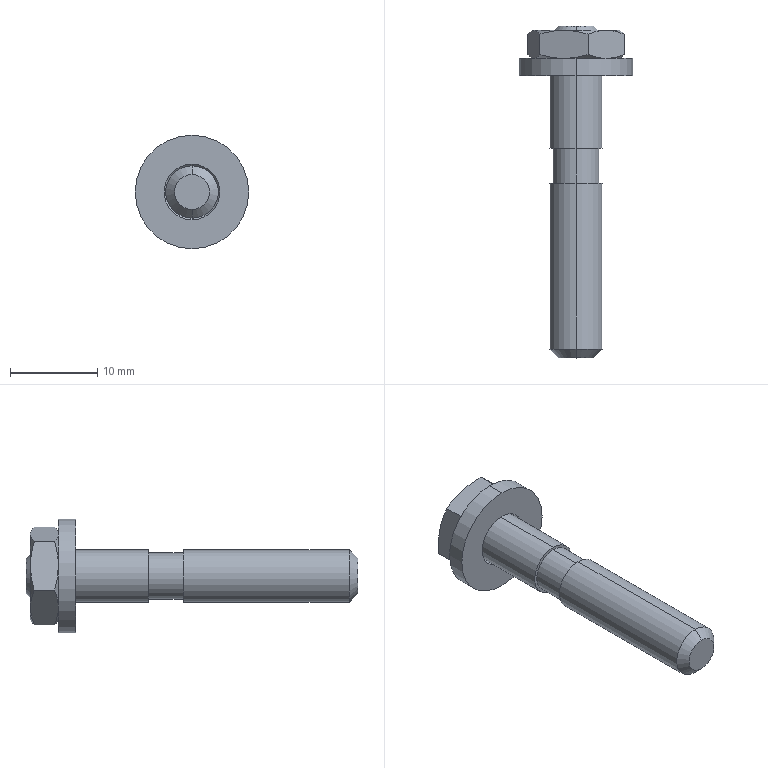Part | SolidWorks | features BaseBody 1 | 1 solid | 49 faces | box 13 x 38 x 13 mm | volume 1413 mm3 | cone 25 | plane 14 | cylinder 10 | commonest cylinder face diameters 6 x4 5.3 x2 6.4 x2 13 x2
STEP:
#1=CARTESIAN_POINT('',(13.099,44.62,-33.));
#2=VERTEX_POINT('',#1);
#3=CARTESIAN_POINT('',(13.099,44.62,-27.));
#4=VERTEX_POINT('',#3);
#5=CARTESIAN_POINT('',(13.099,44.62,-30.));
#6=DIRECTION('',(0.,-1.,0.));
#7=DIRECTION('',(0.,0.,-1.));
#8=AXIS2_PLACEMENT_3D('',#5,#6,#7);
#9=CIRCLE('',#8,3.);
#10=EDGE_CURVE('',#2,#4,#9,.T.);
#11=ORIENTED_EDGE('',*,*,#10,.T.);
#12=CARTESIAN_POINT('',(13.099,25.62,-27.));
#13=VERTEX_POINT('',#12);
#14=CARTESIAN_POINT('',(13.099,44.62,-27.));
#15=DIRECTION('',(0.,-1.,0.));
#16=VECTOR('',#15,1000.);
#17=LINE('',#14,#16);
#18=EDGE_CURVE('',#4,#13,#17,.T.);
#19=ORIENTED_EDGE('',*,*,#18,.T.);
#20=CARTESIAN_POINT('',(13.099,25.62,-33.));
#21=VERTEX_POINT('',#20);
#22=CARTESIAN_POINT('',(13.099,25.62,-30.));
#23=DIRECTION('',(0.,1.,0.));
#24=DIRECTION('',(0.,0.,-1.));
#25=AXIS2_PLACEMENT_3D('',#22,#23,#24);
#26=CIRCLE('',#25,3.);
#27=EDGE_CURVE('',#13,#21,#26,.T.);
#28=ORIENTED_EDGE('',*,*,#27,.T.);
#29=CARTESIAN_POINT('',(13.099,44.62,-33.));
#30=DIRECTION('',(0.,-1.,0.));
#31=VECTOR('',#30,1000.);
#32=LINE('',#29,#31);
#33=EDGE_CURVE('',#2,#21,#32,.T.);
#34=ORIENTED_EDGE('',*,*,#33,.F.);
#35=EDGE_LOOP('',(#11,#19,#28,#34));
#36=FACE_OUTER_BOUND('',#35,.T.);
#37=CARTESIAN_POINT('',(13.099,44.62,-30.));
#38=DIRECTION('',(0.,-1.,0.));
#39=DIRECTION('',(0.,0.,-1.));
#40=AXIS2_PLACEMENT_3D('',#37,#38,#39);
#41=CYLINDRICAL_SURFACE('',#40,3.);
#42=ADVANCED_FACE('',(#36),#41,.T.);
#43=CARTESIAN_POINT('',(13.099,24.62,-28.));
#44=VERTEX_POINT('',#43);
#45=CARTESIAN_POINT('',(13.099,24.62,-32.));
#46=VERTEX_POINT('',#45);
#47=CARTESIAN_POINT('',(13.099,24.62,-30.));
#48=DIRECTION('',(0.,1.,0.));
#49=DIRECTION('',(0.,0.,1.));
#50=AXIS2_PLACEMENT_3D('',#47,#48,#49);
#51=CIRCLE('',#50,2.);
#52=EDGE_CURVE('',#44,#46,#51,.T.);
#53=ORIENTED_EDGE('',*,*,#52,.T.);
#54=CARTESIAN_POINT('',(13.099,25.62,-33.));
#55=DIRECTION('',(0.,0.7071,-0.7071));
#56=VECTOR('',#55,1000.);
#57=LINE('',#54,#56);
#58=EDGE_CURVE('',#46,#21,#57,.T.);
#59=ORIENTED_EDGE('',*,*,#58,.T.);
#60=ORIENTED_EDGE('',*,*,#27,.F.);
#61=CARTESIAN_POINT('',(13.099,25.62,-27.));
#62=DIRECTION('',(0.,0.7071,0.7071));
#63=VECTOR('',#62,1000.);
#64=LINE('',#61,#63);
#65=EDGE_CURVE('',#44,#13,#64,.T.);
#66=ORIENTED_EDGE('',*,*,#65,.F.);
#67=EDGE_LOOP('',(#53,#59,#60,#66));
#68=FACE_OUTER_BOUND('',#67,.T.);
#69=CARTESIAN_POINT('',(13.099,25.62,-30.));
#70=DIRECTION('',(0.,1.,0.));
#71=DIRECTION('',(0.,0.,1.));
#72=AXIS2_PLACEMENT_3D('',#69,#70,#71);
#73=CONICAL_SURFACE('',#72,3.,0.7854);
#74=ADVANCED_FACE('',(#68),#73,.T.);
#75=CARTESIAN_POINT('',(13.099,48.62,-32.65));
#76=VERTEX_POINT('',#75);
#77=CARTESIAN_POINT('',(13.099,48.62,-27.35));
#78=VERTEX_POINT('',#77);
#79=CARTESIAN_POINT('',(13.099,48.62,-30.));
#80=DIRECTION('',(0.,-1.,0.));
#81=DIRECTION('',(0.,0.,-1.));
#82=AXIS2_PLACEMENT_3D('',#79,#80,#81);
#83=CIRCLE('',#82,2.65);
#84=EDGE_CURVE('',#76,#78,#83,.T.);
#85=ORIENTED_EDGE('',*,*,#84,.T.);
#86=CARTESIAN_POINT('',(13.099,44.62,-27.35));
#87=VERTEX_POINT('',#86);
#88=CARTESIAN_POINT('',(13.099,48.62,-27.35));
#89=DIRECTION('',(0.,-1.,0.));
#90=VECTOR('',#89,1000.);
#91=LINE('',#88,#90);
#92=EDGE_CURVE('',#78,#87,#91,.T.);
#93=ORIENTED_EDGE('',*,*,#92,.T.);
#94=CARTESIAN_POINT('',(13.099,44.62,-32.65));
#95=VERTEX_POINT('',#94);
#96=CARTESIAN_POINT('',(13.099,44.62,-30.));
#97=DIRECTION('',(0.,-1.,0.));
#98=DIRECTION('',(0.,0.,-1.));
#99=AXIS2_PLACEMENT_3D('',#96,#97,#98);
#100=CIRCLE('',#99,2.65);
#101=EDGE_CURVE('',#95,#87,#100,.T.);
#102=ORIENTED_EDGE('',*,*,#101,.F.);
#103=CARTESIAN_POINT('',(13.099,48.62,-32.65));
#104=DIRECTION('',(0.,-1.,0.));
#105=VECTOR('',#104,1000.);
#106=LINE('',#103,#105);
#107=EDGE_CURVE('',#76,#95,#106,.T.);
#108=ORIENTED_EDGE('',*,*,#107,.F.);
#109=EDGE_LOOP('',(#85,#93,#102,#108));
#110=FACE_OUTER_BOUND('',#109,.T.);
#111=CARTESIAN_POINT('',(13.099,48.62,-30.));
#112=DIRECTION('',(0.,-1.,0.));
#113=DIRECTION('',(0.,0.,-1.));
#114=AXIS2_PLACEMENT_3D('',#111,#112,#113);
#115=CYLINDRICAL_SURFACE('',#114,2.65);
#116=ADVANCED_FACE('',(#110),#115,.T.);
#117=CARTESIAN_POINT('',(13.099,59.42,-33.));
#118=VERTEX_POINT('',#117);
#119=CARTESIAN_POINT('',(13.099,59.42,-27.));
#120=VERTEX_POINT('',#119);
#121=CARTESIAN_POINT('',(13.099,59.42,-30.));
#122=DIRECTION('',(0.,-1.,0.));
#123=DIRECTION('',(0.,0.,-1.));
#124=AXIS2_PLACEMENT_3D('',#121,#122,#123);
#125=CIRCLE('',#124,3.);
#126=EDGE_CURVE('',#118,#120,#125,.T.);
#127=ORIENTED_EDGE('',*,*,#126,.T.);
#128=CARTESIAN_POINT('',(13.099,48.62,-27.));
#129=VERTEX_POINT('',#128);
#130=CARTESIAN_POINT('',(13.099,59.42,-27.));
#131=DIRECTION('',(0.,-1.,0.));
#132=VECTOR('',#131,1000.);
#133=LINE('',#130,#132);
#134=EDGE_CURVE('',#120,#129,#133,.T.);
#135=ORIENTED_EDGE('',*,*,#134,.T.);
#136=CARTESIAN_POINT('',(13.099,48.62,-33.));
#137=VERTEX_POINT('',#136);
#138=CARTESIAN_POINT('',(13.099,48.62,-30.));
#139=DIRECTION('',(0.,1.,0.));
#140=DIRECTION('',(0.,0.,-1.));
#141=AXIS2_PLACEMENT_3D('',#138,#139,#140);
#142=CIRCLE('',#141,3.);
#143=EDGE_CURVE('',#129,#137,#142,.T.);
#144=ORIENTED_EDGE('',*,*,#143,.T.);
#145=CARTESIAN_POINT('',(13.099,59.42,-33.));
#146=DIRECTION('',(0.,-1.,0.));
#147=VECTOR('',#146,1000.);
#148=LINE('',#145,#147);
#149=EDGE_CURVE('',#118,#137,#148,.T.);
#150=ORIENTED_EDGE('',*,*,#149,.F.);
#151=EDGE_LOOP('',(#127,#135,#144,#150));
#152=FACE_OUTER_BOUND('',#151,.T.);
#153=CARTESIAN_POINT('',(13.099,59.42,-30.));
#154=DIRECTION('',(0.,-1.,0.));
#155=DIRECTION('',(0.,0.,-1.));
#156=AXIS2_PLACEMENT_3D('',#153,#154,#155);
#157=CYLINDRICAL_SURFACE('',#156,3.);
#158=ADVANCED_FACE('',(#152),#157,.T.);
#159=CARTESIAN_POINT('',(13.099,59.42,-30.));
#160=DIRECTION('',(0.,-1.,0.));
#161=DIRECTION('',(0.,0.,-1.));
#162=AXIS2_PLACEMENT_3D('',#159,#160,#161);
#163=CIRCLE('',#162,3.);
#164=EDGE_CURVE('',#120,#118,#163,.T.);
#165=ORIENTED_EDGE('',*,*,#164,.F.);
#166=CARTESIAN_POINT('',(13.099,58.92,-26.5));
#167=VERTEX_POINT('',#166);
#168=CARTESIAN_POINT('',(13.099,58.92,-26.5));
#169=DIRECTION('',(0.,-0.7071,0.7071));
#170=VECTOR('',#169,1000.);
#171=LINE('',#168,#170);
#172=EDGE_CURVE('',#120,#167,#171,.T.);
#173=ORIENTED_EDGE('',*,*,#172,.T.);
#174=CARTESIAN_POINT('',(13.099,58.92,-33.5));
#175=VERTEX_POINT('',#174);
#176=CARTESIAN_POINT('',(13.099,58.92,-30.));
#177=DIRECTION('',(0.,1.,0.));
#178=DIRECTION('',(0.,0.,-1.));
#179=AXIS2_PLACEMENT_3D('',#176,#177,#178);
#180=CIRCLE('',#179,3.5);
#181=EDGE_CURVE('',#175,#167,#180,.T.);
#182=ORIENTED_EDGE('',*,*,#181,.F.);
#183=CARTESIAN_POINT('',(13.099,58.92,-33.5));
#184=DIRECTION('',(0.,-0.7071,-0.7071));
#185=VECTOR('',#184,1000.);
#186=LINE('',#183,#185);
#187=EDGE_CURVE('',#118,#175,#186,.T.);
#188=ORIENTED_EDGE('',*,*,#187,.F.);
#189=EDGE_LOOP('',(#165,#173,#182,#188));
#190=FACE_OUTER_BOUND('',#189,.T.);
#191=CARTESIAN_POINT('',(13.099,58.92,-30.));
#192=DIRECTION('',(0.,-1.,0.));
#193=DIRECTION('',(0.,0.,-1.));
#194=AXIS2_PLACEMENT_3D('',#191,#192,#193);
#195=CONICAL_SURFACE('',#194,3.5,0.7854);
#196=ADVANCED_FACE('',(#190),#195,.F.);
#197=CARTESIAN_POINT('',(13.099,56.92,-33.2));
#198=VERTEX_POINT('',#197);
#199=CARTESIAN_POINT('',(13.099,56.92,-26.8));
#200=VERTEX_POINT('',#199);
#201=CARTESIAN_POINT('',(13.099,56.92,-30.));
#202=DIRECTION('',(0.,1.,0.));
#203=DIRECTION('',(0.,0.,1.));
#204=AXIS2_PLACEMENT_3D('',#201,#202,#203);
#205=CIRCLE('',#204,3.2);
#206=EDGE_CURVE('',#198,#200,#205,.T.);
#207=ORIENTED_EDGE('',*,*,#206,.F.);
#208=CARTESIAN_POINT('',(13.099,58.92,-33.2));
#209=VERTEX_POINT('',#208);
#210=CARTESIAN_POINT('',(13.099,56.92,-33.2));
#211=DIRECTION('',(0.,1.,0.));
#212=VECTOR('',#211,1000.);
#213=LINE('',#210,#212);
#214=EDGE_CURVE('',#198,#209,#213,.T.);
#215=ORIENTED_EDGE('',*,*,#214,.T.);
#216=CARTESIAN_POINT('',(13.099,58.92,-26.8));
#217=VERTEX_POINT('',#216);
#218=CARTESIAN_POINT('',(13.099,58.92,-30.));
#219=DIRECTION('',(0.,-1.,0.));
#220=DIRECTION('',(0.,0.,1.));
#221=AXIS2_PLACEMENT_3D('',#218,#219,#220);
#222=CIRCLE('',#221,3.2);
#223=EDGE_CURVE('',#217,#209,#222,.T.);
#224=ORIENTED_EDGE('',*,*,#223,.F.);
#225=CARTESIAN_POINT('',(13.099,56.92,-26.8));
#226=DIRECTION('',(0.,1.,0.));
#227=VECTOR('',#226,1000.);
#228=LINE('',#225,#227);
#229=EDGE_CURVE('',#200,#217,#228,.T.);
#230=ORIENTED_EDGE('',*,*,#229,.F.);
#231=EDGE_LOOP('',(#207,#215,#224,#230));
#232=FACE_OUTER_BOUND('',#231,.T.);
#233=CARTESIAN_POINT('',(13.099,56.92,-30.));
#234=DIRECTION('',(0.,1.,0.));
#235=DIRECTION('',(0.,0.,1.));
#236=AXIS2_PLACEMENT_3D('',#233,#234,#235);
#237=CYLINDRICAL_SURFACE('',#236,3.2);
#238=ADVANCED_FACE('',(#232),#237,.F.);
#239=CARTESIAN_POINT('',(13.099,56.92,-23.5));
#240=VERTEX_POINT('',#239);
#241=CARTESIAN_POINT('',(13.099,56.92,-36.5));
#242=VERTEX_POINT('',#241);
#243=CARTESIAN_POINT('',(13.099,56.92,-30.));
#244=DIRECTION('',(0.,1.,0.));
#245=DIRECTION('',(0.,0.,1.));
#246=AXIS2_PLACEMENT_3D('',#243,#244,#245);
#247=CIRCLE('',#246,6.5);
#248=EDGE_CURVE('',#240,#242,#247,.T.);
#249=ORIENTED_EDGE('',*,*,#248,.T.);
#250=CARTESIAN_POINT('',(13.099,58.92,-36.5));
#251=VERTEX_POINT('',#250);
#252=CARTESIAN_POINT('',(13.099,56.92,-36.5));
#253=DIRECTION('',(0.,1.,0.));
#254=VECTOR('',#253,1000.);
#255=LINE('',#252,#254);
#256=EDGE_CURVE('',#242,#251,#255,.T.);
#257=ORIENTED_EDGE('',*,*,#256,.T.);
#258=CARTESIAN_POINT('',(13.099,58.92,-23.5));
#259=VERTEX_POINT('',#258);
#260=CARTESIAN_POINT('',(13.099,58.92,-30.));
#261=DIRECTION('',(0.,-1.,0.));
#262=DIRECTION('',(0.,0.,1.));
#263=AXIS2_PLACEMENT_3D('',#260,#261,#262);
#264=CIRCLE('',#263,6.5);
#265=EDGE_CURVE('',#251,#259,#264,.T.);
#266=ORIENTED_EDGE('',*,*,#265,.T.);
#267=CARTESIAN_POINT('',(13.099,56.92,-23.5));
#268=DIRECTION('',(0.,1.,0.));
#269=VECTOR('',#268,1000.);
#270=LINE('',#267,#269);
#271=EDGE_CURVE('',#240,#259,#270,.T.);
#272=ORIENTED_EDGE('',*,*,#271,.F.);
#273=EDGE_LOOP('',(#249,#257,#266,#272));
#274=FACE_OUTER_BOUND('',#273,.T.);
#275=CARTESIAN_POINT('',(13.099,56.92,-30.));
#276=DIRECTION('',(0.,1.,0.));
#277=DIRECTION('',(0.,0.,1.));
#278=AXIS2_PLACEMENT_3D('',#275,#276,#277);
#279=CYLINDRICAL_SURFACE('',#278,6.5);
#280=ADVANCED_FACE('',(#274),#279,.T.);
#281=CARTESIAN_POINT('',(13.099,61.62,-33.));
#282=VERTEX_POINT('',#281);
#283=CARTESIAN_POINT('',(13.099,61.62,-27.));
#284=VERTEX_POINT('',#283);
#285=CARTESIAN_POINT('',(13.099,61.62,-30.));
#286=DIRECTION('',(0.,1.,0.));
#287=DIRECTION('',(0.,0.,1.));
#288=AXIS2_PLACEMENT_3D('',#285,#286,#287);
#289=CIRCLE('',#288,3.);
#290=EDGE_CURVE('',#282,#284,#289,.T.);
#291=ORIENTED_EDGE('',*,*,#290,.F.);
#292=CARTESIAN_POINT('',(13.099,62.12,-33.5));
#293=VERTEX_POINT('',#292);
#294=CARTESIAN_POINT('',(13.099,62.12,-33.5));
#295=DIRECTION('',(0.,0.7071,-0.7071));
#296=VECTOR('',#295,1000.);
#297=LINE('',#294,#296);
#298=EDGE_CURVE('',#282,#293,#297,.T.);
#299=ORIENTED_EDGE('',*,*,#298,.T.);
#300=CARTESIAN_POINT('',(13.099,62.12,-26.5));
#301=VERTEX_POINT('',#300);
#302=CARTESIAN_POINT('',(13.099,62.12,-30.));
#303=DIRECTION('',(0.,-1.,0.));
#304=DIRECTION('',(0.,0.,1.));
#305=AXIS2_PLACEMENT_3D('',#302,#303,#304);
#306=CIRCLE('',#305,3.5);
#307=EDGE_CURVE('',#301,#293,#306,.T.);
#308=ORIENTED_EDGE('',*,*,#307,.F.);
#309=CARTESIAN_POINT('',(13.099,62.12,-26.5));
#310=DIRECTION('',(0.,0.7071,0.7071));
#311=VECTOR('',#310,1000.);
#312=LINE('',#309,#311);
#313=EDGE_CURVE('',#284,#301,#312,.T.);
#314=ORIENTED_EDGE('',*,*,#313,.F.);
#315=EDGE_LOOP('',(#291,#299,#308,#314));
#316=FACE_OUTER_BOUND('',#315,.T.);
#317=CARTESIAN_POINT('',(13.099,62.12,-30.));
#318=DIRECTION('',(0.,1.,0.));
#319=DIRECTION('',(0.,0.,1.));
#320=AXIS2_PLACEMENT_3D('',#317,#318,#319);
#321=CONICAL_SURFACE('',#320,3.5,0.7854);
#322=ADVANCED_FACE('',(#316),#321,.F.);
#323=CARTESIAN_POINT('',(13.099,62.62,-32.));
#324=VERTEX_POINT('',#323);
#325=CARTESIAN_POINT('',(13.099,62.62,-28.));
#326=VERTEX_POINT('',#325);
#327=CARTESIAN_POINT('',(13.099,62.62,-30.));
#328=DIRECTION('',(0.,-1.,0.));
#329=DIRECTION('',(0.,0.,-1.));
#330=AXIS2_PLACEMENT_3D('',#327,#328,#329);
#331=CIRCLE('',#330,2.);
#332=EDGE_CURVE('',#324,#326,#331,.T.);
#333=ORIENTED_EDGE('',*,*,#332,.T.);
#334=CARTESIAN_POINT('',(13.099,61.62,-27.));
#335=DIRECTION('',(0.,-0.7071,0.7071));
#336=VECTOR('',#335,1000.);
#337=LINE('',#334,#336);
#338=EDGE_CURVE('',#326,#284,#337,.T.);
#339=ORIENTED_EDGE('',*,*,#338,.T.);
#340=CARTESIAN_POINT('',(13.099,61.62,-30.));
#341=DIRECTION('',(0.,1.,0.));
#342=DIRECTION('',(0.,0.,1.));
#343=AXIS2_PLACEMENT_3D('',#340,#341,#342);
#344=CIRCLE('',#343,3.);
#345=EDGE_CURVE('',#284,#282,#344,.T.);
#346=ORIENTED_EDGE('',*,*,#345,.T.);
#347=CARTESIAN_POINT('',(13.099,61.62,-33.));
#348=DIRECTION('',(0.,-0.7071,-0.7071));
#349=VECTOR('',#348,1000.);
#350=LINE('',#347,#349);
#351=EDGE_CURVE('',#324,#282,#350,.T.);
#352=ORIENTED_EDGE('',*,*,#351,.F.);
#353=EDGE_LOOP('',(#333,#339,#346,#352));
#354=FACE_OUTER_BOUND('',#353,.T.);
#355=CARTESIAN_POINT('',(13.099,61.62,-30.));
#356=DIRECTION('',(0.,-1.,0.));
#357=DIRECTION('',(0.,0.,-1.));
#358=AXIS2_PLACEMENT_3D('',#355,#356,#357);
#359=CONICAL_SURFACE('',#358,3.,0.7854);
#360=ADVANCED_FACE('',(#354),#359,.T.);
#361=ORIENTED_EDGE('',*,*,#18,.F.);
#362=CARTESIAN_POINT('',(13.099,44.62,-30.));
#363=DIRECTION('',(0.,-1.,0.));
#364=DIRECTION('',(0.,0.,-1.));
#365=AXIS2_PLACEMENT_3D('',#362,#363,#364);
#366=CIRCLE('',#365,3.);
#367=EDGE_CURVE('',#4,#2,#366,.T.);
#368=ORIENTED_EDGE('',*,*,#367,.T.);
#369=ORIENTED_EDGE('',*,*,#33,.T.);
#370=CARTESIAN_POINT('',(13.099,25.62,-30.));
#371=DIRECTION('',(0.,1.,0.));
#372=DIRECTION('',(0.,0.,-1.));
#373=AXIS2_PLACEMENT_3D('',#370,#371,#372);
#374=CIRCLE('',#373,3.);
#375=EDGE_CURVE('',#21,#13,#374,.T.);
#376=ORIENTED_EDGE('',*,*,#375,.T.);
#377=EDGE_LOOP('',(#361,#368,#369,#376));
#378=FACE_OUTER_BOUND('',#377,.T.);
#379=CARTESIAN_POINT('',(13.099,44.62,-30.));
#380=DIRECTION('',(0.,-1.,0.));
#381=DIRECTION('',(0.,0.,-1.));
#382=AXIS2_PLACEMENT_3D('',#379,#380,#381);
#383=CYLINDRICAL_SURFACE('',#382,3.);
#384=ADVANCED_FACE('',(#378),#383,.T.);
#385=ORIENTED_EDGE('',*,*,#101,.T.);
#386=CARTESIAN_POINT('',(13.099,44.62,-30.));
#387=DIRECTION('',(0.,-1.,0.));
#388=DIRECTION('',(0.,0.,-1.));
#389=AXIS2_PLACEMENT_3D('',#386,#387,#388);
#390=CIRCLE('',#389,2.65);
#391=EDGE_CURVE('',#87,#95,#390,.T.);
#392=ORIENTED_EDGE('',*,*,#391,.T.);
#393=EDGE_LOOP('',(#385,#392));
#394=FACE_BOUND('',#393,.T.);
#395=ORIENTED_EDGE('',*,*,#10,.F.);
#396=ORIENTED_EDGE('',*,*,#367,.F.);
#397=EDGE_LOOP('',(#395,#396));
#398=FACE_OUTER_BOUND('',#397,.T.);
#399=CARTESIAN_POINT('',(13.099,44.62,-30.));
#400=DIRECTION('',(0.,1.,0.));
#401=DIRECTION('',(0.,0.,1.));
#402=AXIS2_PLACEMENT_3D('',#399,#400,#401);
#403=PLANE('',#402);
#404=ADVANCED_FACE('',(#394,#398),#403,.T.);
#405=ORIENTED_EDGE('',*,*,#58,.F.);
#406=CARTESIAN_POINT('',(13.099,24.62,-30.));
#407=DIRECTION('',(0.,1.,0.));
#408=DIRECTION('',(0.,0.,1.));
#409=AXIS2_PLACEMENT_3D('',#406,#407,#408);
#410=CIRCLE('',#409,2.);
#411=EDGE_CURVE('',#46,#44,#410,.T.);
#412=ORIENTED_EDGE('',*,*,#411,.T.);
#413=ORIENTED_EDGE('',*,*,#65,.T.);
#414=ORIENTED_EDGE('',*,*,#375,.F.);
#415=EDGE_LOOP('',(#405,#412,#413,#414));
#416=FACE_OUTER_BOUND('',#415,.T.);
#417=CARTESIAN_POINT('',(13.099,25.62,-30.));
#418=DIRECTION('',(0.,1.,0.));
#419=DIRECTION('',(0.,0.,1.));
#420=AXIS2_PLACEMENT_3D('',#417,#418,#419);
#421=CONICAL_SURFACE('',#420,3.,0.7854);
#422=ADVANCED_FACE('',(#416),#421,.T.);
#423=ORIENTED_EDGE('',*,*,#92,.F.);
#424=CARTESIAN_POINT('',(13.099,48.62,-30.));
#425=DIRECTION('',(0.,-1.,0.));
#426=DIRECTION('',(0.,0.,-1.));
#427=AXIS2_PLACEMENT_3D('',#424,#425,#426);
#428=CIRCLE('',#427,2.65);
#429=EDGE_CURVE('',#78,#76,#428,.T.);
#430=ORIENTED_EDGE('',*,*,#429,.T.);
#431=ORIENTED_EDGE('',*,*,#107,.T.);
#432=ORIENTED_EDGE('',*,*,#391,.F.);
#433=EDGE_LOOP('',(#423,#430,#431,#432));
#434=FACE_OUTER_BOUND('',#433,.T.);
#435=CARTESIAN_POINT('',(13.099,48.62,-30.));
#436=DIRECTION('',(0.,-1.,0.));
#437=DIRECTION('',(0.,0.,-1.));
#438=AXIS2_PLACEMENT_3D('',#435,#436,#437);
#439=CYLINDRICAL_SURFACE('',#438,2.65);
#440=ADVANCED_FACE('',(#434),#439,.T.);
#441=ORIENTED_EDGE('',*,*,#52,.F.);
#442=ORIENTED_EDGE('',*,*,#411,.F.);
#443=EDGE_LOOP('',(#441,#442));
#444=FACE_OUTER_BOUND('',#443,.T.);
#445=CARTESIAN_POINT('',(13.099,24.62,-30.));
#446=DIRECTION('',(0.,1.,0.));
#447=DIRECTION('',(0.,0.,1.));
#448=AXIS2_PLACEMENT_3D('',#445,#446,#447);
#449=PLANE('',#448);
#450=ADVANCED_FACE('',(#444),#449,.F.);
#451=ORIENTED_EDGE('',*,*,#84,.F.);
#452=ORIENTED_EDGE('',*,*,#429,.F.);
#453=EDGE_LOOP('',(#451,#452));
#454=FACE_BOUND('',#453,.T.);
#455=CARTESIAN_POINT('',(13.099,48.62,-30.));
#456=DIRECTION('',(0.,1.,0.));
#457=DIRECTION('',(0.,0.,-1.));
#458=AXIS2_PLACEMENT_3D('',#455,#456,#457);
#459=CIRCLE('',#458,3.);
#460=EDGE_CURVE('',#137,#129,#459,.T.);
#461=ORIENTED_EDGE('',*,*,#460,.F.);
#462=ORIENTED_EDGE('',*,*,#143,.F.);
#463=EDGE_LOOP('',(#461,#462));
#464=FACE_OUTER_BOUND('',#463,.T.);
#465=CARTESIAN_POINT('',(13.099,48.62,-30.));
#466=DIRECTION('',(0.,1.,0.));
#467=DIRECTION('',(0.,0.,1.));
#468=AXIS2_PLACEMENT_3D('',#465,#466,#467);
#469=PLANE('',#468);
#470=ADVANCED_FACE('',(#454,#464),#469,.F.);
#471=ORIENTED_EDGE('',*,*,#134,.F.);
#472=ORIENTED_EDGE('',*,*,#164,.T.);
#473=ORIENTED_EDGE('',*,*,#149,.T.);
#474=ORIENTED_EDGE('',*,*,#460,.T.);
#475=EDGE_LOOP('',(#471,#472,#473,#474));
#476=FACE_OUTER_BOUND('',#475,.T.);
#477=CARTESIAN_POINT('',(13.099,59.42,-30.));
#478=DIRECTION('',(0.,-1.,0.));
#479=DIRECTION('',(0.,0.,-1.));
#480=AXIS2_PLACEMENT_3D('',#477,#478,#479);
#481=CYLINDRICAL_SURFACE('',#480,3.);
#482=ADVANCED_FACE('',(#476),#481,.T.);
#483=ORIENTED_EDGE('',*,*,#172,.F.);
#484=ORIENTED_EDGE('',*,*,#126,.F.);
#485=ORIENTED_EDGE('',*,*,#187,.T.);
#486=CARTESIAN_POINT('',(13.099,58.92,-30.));
#487=DIRECTION('',(0.,1.,0.));
#488=DIRECTION('',(0.,0.,-1.));
#489=AXIS2_PLACEMENT_3D('',#486,#487,#488);
#490=CIRCLE('',#489,3.5);
#491=EDGE_CURVE('',#167,#175,#490,.T.);
#492=ORIENTED_EDGE('',*,*,#491,.F.);
#493=EDGE_LOOP('',(#483,#484,#485,#492));
#494=FACE_OUTER_BOUND('',#493,.T.);
#495=CARTESIAN_POINT('',(13.099,58.92,-30.));
#496=DIRECTION('',(0.,-1.,0.));
#497=DIRECTION('',(0.,0.,-1.));
#498=AXIS2_PLACEMENT_3D('',#495,#496,#497);
#499=CONICAL_SURFACE('',#498,3.5,0.7854);
#500=ADVANCED_FACE('',(#494),#499,.F.);
#501=ORIENTED_EDGE('',*,*,#223,.T.);
#502=CARTESIAN_POINT('',(13.099,58.92,-30.));
#503=DIRECTION('',(0.,-1.,0.));
#504=DIRECTION('',(0.,0.,1.));
#505=AXIS2_PLACEMENT_3D('',#502,#503,#504);
#506=CIRCLE('',#505,3.2);
#507=EDGE_CURVE('',#209,#217,#506,.T.);
#508=ORIENTED_EDGE('',*,*,#507,.T.);
#509=EDGE_LOOP('',(#501,#508));
#510=FACE_BOUND('',#509,.T.);
#511=ORIENTED_EDGE('',*,*,#181,.T.);
#512=ORIENTED_EDGE('',*,*,#491,.T.);
#513=EDGE_LOOP('',(#511,#512));
#514=FACE_OUTER_BOUND('',#513,.T.);
#515=CARTESIAN_POINT('',(13.099,58.92,-30.));
#516=DIRECTION('',(0.,1.,0.));
#517=DIRECTION('',(0.,0.,1.));
#518=AXIS2_PLACEMENT_3D('',#515,#516,#517);
#519=PLANE('',#518);
#520=ADVANCED_FACE('',(#510,#514),#519,.T.);
#521=ORIENTED_EDGE('',*,*,#214,.F.);
#522=CARTESIAN_POINT('',(13.099,56.92,-30.));
#523=DIRECTION('',(0.,1.,0.));
#524=DIRECTION('',(0.,0.,1.));
#525=AXIS2_PLACEMENT_3D('',#522,#523,#524);
#526=CIRCLE('',#525,3.2);
#527=EDGE_CURVE('',#200,#198,#526,.T.);
#528=ORIENTED_EDGE('',*,*,#527,.F.);
#529=ORIENTED_EDGE('',*,*,#229,.T.);
#530=ORIENTED_EDGE('',*,*,#507,.F.);
#531=EDGE_LOOP('',(#521,#528,#529,#530));
#532=FACE_OUTER_BOUND('',#531,.T.);
#533=CARTESIAN_POINT('',(13.099,56.92,-30.));
#534=DIRECTION('',(0.,1.,0.));
#535=DIRECTION('',(0.,0.,1.));
#536=AXIS2_PLACEMENT_3D('',#533,#534,#535);
#537=CYLINDRICAL_SURFACE('',#536,3.2);
#538=ADVANCED_FACE('',(#532),#537,.F.);
#539=ORIENTED_EDGE('',*,*,#527,.T.);
#540=ORIENTED_EDGE('',*,*,#206,.T.);
#541=EDGE_LOOP('',(#539,#540));
#542=FACE_BOUND('',#541,.T.);
#543=ORIENTED_EDGE('',*,*,#248,.F.);
#544=CARTESIAN_POINT('',(13.099,56.92,-30.));
#545=DIRECTION('',(0.,1.,0.));
#546=DIRECTION('',(0.,0.,1.));
#547=AXIS2_PLACEMENT_3D('',#544,#545,#546);
#548=CIRCLE('',#547,6.5);
#549=EDGE_CURVE('',#242,#240,#548,.T.);
#550=ORIENTED_EDGE('',*,*,#549,.F.);
#551=EDGE_LOOP('',(#543,#550));
#552=FACE_OUTER_BOUND('',#551,.T.);
#553=CARTESIAN_POINT('',(13.099,56.92,-30.));
#554=DIRECTION('',(0.,1.,0.));
#555=DIRECTION('',(0.,0.,1.));
#556=AXIS2_PLACEMENT_3D('',#553,#554,#555);
#557=PLANE('',#556);
#558=ADVANCED_FACE('',(#542,#552),#557,.F.);
#559=ORIENTED_EDGE('',*,*,#256,.F.);
#560=ORIENTED_EDGE('',*,*,#549,.T.);
#561=ORIENTED_EDGE('',*,*,#271,.T.);
#562=CARTESIAN_POINT('',(13.099,58.92,-30.));
#563=DIRECTION('',(0.,-1.,0.));
#564=DIRECTION('',(0.,0.,1.));
#565=AXIS2_PLACEMENT_3D('',#562,#563,#564);
#566=CIRCLE('',#565,6.5);
#567=EDGE_CURVE('',#259,#251,#566,.T.);
#568=ORIENTED_EDGE('',*,*,#567,.T.);
#569=EDGE_LOOP('',(#559,#560,#561,#568));
#570=FACE_OUTER_BOUND('',#569,.T.);
#571=CARTESIAN_POINT('',(13.099,56.92,-30.));
#572=DIRECTION('',(0.,1.,0.));
#573=DIRECTION('',(0.,0.,1.));
#574=AXIS2_PLACEMENT_3D('',#571,#572,#573);
#575=CYLINDRICAL_SURFACE('',#574,6.5);
#576=ADVANCED_FACE('',(#570),#575,.T.);
#577=CARTESIAN_POINT('',(8.099,58.92,-30.));
#578=VERTEX_POINT('',#577);
#579=CARTESIAN_POINT('',(9.635,58.92,-33.606));
#580=VERTEX_POINT('',#579);
#581=CARTESIAN_POINT('',(13.099,58.92,-30.));
#582=DIRECTION('',(0.,-1.,0.));
#583=DIRECTION('',(0.,0.,1.));
#584=AXIS2_PLACEMENT_3D('',#581,#582,#583);
#585=CIRCLE('',#584,5.);
#586=EDGE_CURVE('',#578,#580,#585,.T.);
#587=ORIENTED_EDGE('',*,*,#586,.T.);
#588=CARTESIAN_POINT('',(14.49,58.92,-34.803));
#589=VERTEX_POINT('',#588);
#590=CARTESIAN_POINT('',(13.099,58.92,-30.));
#591=DIRECTION('',(0.,-1.,0.));
#592=DIRECTION('',(0.,0.,1.));
#593=AXIS2_PLACEMENT_3D('',#590,#591,#592);
#594=CIRCLE('',#593,5.);
#595=EDGE_CURVE('',#580,#589,#594,.T.);
#596=ORIENTED_EDGE('',*,*,#595,.T.);
#597=CARTESIAN_POINT('',(17.953,58.92,-31.196));
#598=VERTEX_POINT('',#597);
#599=CARTESIAN_POINT('',(13.099,58.92,-30.));
#600=DIRECTION('',(0.,-1.,0.));
#601=DIRECTION('',(0.,0.,1.));
#602=AXIS2_PLACEMENT_3D('',#599,#600,#601);
#603=CIRCLE('',#602,5.);
#604=EDGE_CURVE('',#589,#598,#603,.T.);
#605=ORIENTED_EDGE('',*,*,#604,.T.);
#606=CARTESIAN_POINT('',(16.562,58.92,-26.394));
#607=VERTEX_POINT('',#606);
#608=CARTESIAN_POINT('',(13.099,58.92,-30.));
#609=DIRECTION('',(0.,-1.,0.));
#610=DIRECTION('',(0.,0.,1.));
#611=AXIS2_PLACEMENT_3D('',#608,#609,#610);
#612=CIRCLE('',#611,5.);
#613=EDGE_CURVE('',#598,#607,#612,.T.);
#614=ORIENTED_EDGE('',*,*,#613,.T.);
#615=CARTESIAN_POINT('',(13.099,58.92,-25.));
#616=VERTEX_POINT('',#615);
#617=CARTESIAN_POINT('',(13.099,58.92,-30.));
#618=DIRECTION('',(0.,-1.,0.));
#619=DIRECTION('',(0.,0.,1.));
#620=AXIS2_PLACEMENT_3D('',#617,#618,#619);
#621=CIRCLE('',#620,5.);
#622=EDGE_CURVE('',#607,#616,#621,.T.);
#623=ORIENTED_EDGE('',*,*,#622,.T.);
#624=CARTESIAN_POINT('',(11.707,58.92,-25.197));
#625=VERTEX_POINT('',#624);
#626=CARTESIAN_POINT('',(13.099,58.92,-30.));
#627=DIRECTION('',(0.,-1.,0.));
#628=DIRECTION('',(0.,0.,1.));
#629=AXIS2_PLACEMENT_3D('',#626,#627,#628);
#630=CIRCLE('',#629,5.);
#631=EDGE_CURVE('',#616,#625,#630,.T.);
#632=ORIENTED_EDGE('',*,*,#631,.T.);
#633=CARTESIAN_POINT('',(8.244,58.92,-28.804));
#634=VERTEX_POINT('',#633);
#635=CARTESIAN_POINT('',(13.099,58.92,-30.));
#636=DIRECTION('',(0.,-1.,0.));
#637=DIRECTION('',(0.,0.,1.));
#638=AXIS2_PLACEMENT_3D('',#635,#636,#637);
#639=CIRCLE('',#638,5.);
#640=EDGE_CURVE('',#625,#634,#639,.T.);
#641=ORIENTED_EDGE('',*,*,#640,.T.);
#642=CARTESIAN_POINT('',(13.099,58.92,-30.));
#643=DIRECTION('',(0.,-1.,0.));
#644=DIRECTION('',(0.,0.,1.));
#645=AXIS2_PLACEMENT_3D('',#642,#643,#644);
#646=CIRCLE('',#645,5.);
#647=EDGE_CURVE('',#634,#578,#646,.T.);
#648=ORIENTED_EDGE('',*,*,#647,.T.);
#649=EDGE_LOOP('',(#587,#596,#605,#614,#623,#632,#641,#648));
#650=FACE_BOUND('',#649,.T.);
#651=ORIENTED_EDGE('',*,*,#567,.F.);
#652=ORIENTED_EDGE('',*,*,#265,.F.);
#653=EDGE_LOOP('',(#651,#652));
#654=FACE_OUTER_BOUND('',#653,.T.);
#655=CARTESIAN_POINT('',(13.099,58.92,-30.));
#656=DIRECTION('',(0.,1.,0.));
#657=DIRECTION('',(0.,0.,1.));
#658=AXIS2_PLACEMENT_3D('',#655,#656,#657);
#659=PLANE('',#658);
#660=ADVANCED_FACE('',(#650,#654),#659,.T.);
#661=CARTESIAN_POINT('',(11.717,59.366,-35.606));
#662=VERTEX_POINT('',#661);
#663=CARTESIAN_POINT('',(11.717,59.366,-35.606));
#664=CARTESIAN_POINT('',(12.623,59.094,-35.343));
#665=CARTESIAN_POINT('',(13.544,58.92,-35.077));
#666=CARTESIAN_POINT('',(14.49,58.92,-34.803));
#667=B_SPLINE_CURVE_WITH_KNOTS('',3,(#663,#664,#665,#666),.UNSPECIFIED.,.F.,.F.,(4,4),(0.,0.002921),.UNSPECIFIED.);
#668=EDGE_CURVE('',#662,#589,#667,.T.);
#669=ORIENTED_EDGE('',*,*,#668,.T.);
#670=ORIENTED_EDGE('',*,*,#595,.F.);
#671=CARTESIAN_POINT('',(9.635,58.92,-33.606));
#672=CARTESIAN_POINT('',(10.346,58.92,-34.289));
#673=CARTESIAN_POINT('',(11.037,59.094,-34.952));
#674=CARTESIAN_POINT('',(11.717,59.366,-35.606));
#675=B_SPLINE_CURVE_WITH_KNOTS('',3,(#671,#672,#673,#674),.UNSPECIFIED.,.F.,.F.,(4,4),(0.,0.002921),.UNSPECIFIED.);
#676=EDGE_CURVE('',#580,#662,#675,.T.);
#677=ORIENTED_EDGE('',*,*,#676,.T.);
#678=EDGE_LOOP('',(#669,#670,#677));
#679=FACE_OUTER_BOUND('',#678,.T.);
#680=CARTESIAN_POINT('',(13.099,59.369,-30.));
#681=DIRECTION('',(0.,1.,0.));
#682=DIRECTION('',(0.,0.,1.));
#683=AXIS2_PLACEMENT_3D('',#680,#681,#682);
#684=CONICAL_SURFACE('',#683,5.778,1.047);
#685=ADVANCED_FACE('',(#679),#684,.T.);
#686=CARTESIAN_POINT('',(7.553,59.366,-31.606));
#687=VERTEX_POINT('',#686);
#688=CARTESIAN_POINT('',(7.553,59.366,-31.606));
#689=CARTESIAN_POINT('',(8.233,59.094,-32.26));
#690=CARTESIAN_POINT('',(8.925,58.92,-32.924));
#691=CARTESIAN_POINT('',(9.635,58.92,-33.606));
#692=B_SPLINE_CURVE_WITH_KNOTS('',3,(#688,#689,#690,#691),.UNSPECIFIED.,.F.,.F.,(4,4),(0.,0.002921),.UNSPECIFIED.);
#693=EDGE_CURVE('',#687,#580,#692,.T.);
#694=ORIENTED_EDGE('',*,*,#693,.T.);
#695=ORIENTED_EDGE('',*,*,#586,.F.);
#696=CARTESIAN_POINT('',(7.949,59.006,-30.));
#697=VERTEX_POINT('',#696);
#698=CARTESIAN_POINT('',(8.099,58.92,-30.));
#699=CARTESIAN_POINT('',(7.949,59.006,-30.));
#700=B_SPLINE_CURVE_WITH_KNOTS('',1,(#698,#699),.UNSPECIFIED.,.F.,.F.,(2,2),(0.,1.),.UNSPECIFIED.);
#701=EDGE_CURVE('',#578,#697,#700,.T.);
#702=ORIENTED_EDGE('',*,*,#701,.T.);
#703=CARTESIAN_POINT('',(7.949,59.006,-30.));
#704=CARTESIAN_POINT('',(7.815,59.084,-30.544));
#705=CARTESIAN_POINT('',(7.683,59.209,-31.079));
#706=CARTESIAN_POINT('',(7.553,59.366,-31.606));
#707=B_SPLINE_CURVE_WITH_KNOTS('',3,(#703,#704,#705,#706),.UNSPECIFIED.,.F.,.F.,(4,4),(0.,0.001693),.UNSPECIFIED.);
#708=EDGE_CURVE('',#697,#687,#707,.T.);
#709=ORIENTED_EDGE('',*,*,#708,.T.);
#710=EDGE_LOOP('',(#694,#695,#702,#709));
#711=FACE_OUTER_BOUND('',#710,.T.);
#712=CARTESIAN_POINT('',(13.099,59.369,-30.));
#713=DIRECTION('',(0.,1.,0.));
#714=DIRECTION('',(0.,0.,1.));
#715=AXIS2_PLACEMENT_3D('',#712,#713,#714);
#716=CONICAL_SURFACE('',#715,5.778,1.047);
#717=ADVANCED_FACE('',(#711),#716,.T.);
#718=CARTESIAN_POINT('',(8.244,58.92,-28.804));
#719=CARTESIAN_POINT('',(8.145,58.92,-29.204));
#720=CARTESIAN_POINT('',(8.047,58.95,-29.603));
#721=CARTESIAN_POINT('',(7.949,59.006,-30.));
#722=B_SPLINE_CURVE_WITH_KNOTS('',3,(#718,#719,#720,#721),.UNSPECIFIED.,.F.,.F.,(4,4),(0.,0.001235),.UNSPECIFIED.);
#723=EDGE_CURVE('',#634,#697,#722,.T.);
#724=ORIENTED_EDGE('',*,*,#723,.T.);
#725=ORIENTED_EDGE('',*,*,#701,.F.);
#726=ORIENTED_EDGE('',*,*,#647,.F.);
#727=EDGE_LOOP('',(#724,#725,#726));
#728=FACE_OUTER_BOUND('',#727,.T.);
#729=CARTESIAN_POINT('',(13.099,59.007,-30.));
#730=DIRECTION('',(0.,1.,0.));
#731=DIRECTION('',(0.,0.,1.));
#732=AXIS2_PLACEMENT_3D('',#729,#730,#731);
#733=CONICAL_SURFACE('',#732,5.15,1.047);
#734=ADVANCED_FACE('',(#728),#733,.T.);
#735=CARTESIAN_POINT('',(8.935,59.366,-26.001));
#736=VERTEX_POINT('',#735);
#737=CARTESIAN_POINT('',(8.935,59.366,-26.001));
#738=CARTESIAN_POINT('',(8.709,59.094,-26.916));
#739=CARTESIAN_POINT('',(8.48,58.92,-27.847));
#740=CARTESIAN_POINT('',(8.244,58.92,-28.804));
#741=B_SPLINE_CURVE_WITH_KNOTS('',3,(#737,#738,#739,#740),.UNSPECIFIED.,.F.,.F.,(4,4),(0.,0.002921),.UNSPECIFIED.);
#742=EDGE_CURVE('',#736,#634,#741,.T.);
#743=ORIENTED_EDGE('',*,*,#742,.T.);
#744=ORIENTED_EDGE('',*,*,#640,.F.);
#745=CARTESIAN_POINT('',(11.707,58.92,-25.197));
#746=CARTESIAN_POINT('',(10.761,58.92,-25.472));
#747=CARTESIAN_POINT('',(9.841,59.094,-25.738));
#748=CARTESIAN_POINT('',(8.935,59.366,-26.001));
#749=B_SPLINE_CURVE_WITH_KNOTS('',3,(#745,#746,#747,#748),.UNSPECIFIED.,.F.,.F.,(4,4),(0.,0.002921),.UNSPECIFIED.);
#750=EDGE_CURVE('',#625,#736,#749,.T.);
#751=ORIENTED_EDGE('',*,*,#750,.T.);
#752=EDGE_LOOP('',(#743,#744,#751));
#753=FACE_OUTER_BOUND('',#752,.T.);
#754=CARTESIAN_POINT('',(13.099,59.369,-30.));
#755=DIRECTION('',(0.,1.,0.));
#756=DIRECTION('',(0.,0.,1.));
#757=AXIS2_PLACEMENT_3D('',#754,#755,#756);
#758=CONICAL_SURFACE('',#757,5.778,1.047);
#759=ADVANCED_FACE('',(#753),#758,.T.);
#760=ORIENTED_EDGE('',*,*,#631,.F.);
#761=CARTESIAN_POINT('',(13.099,59.038,-24.794));
#762=VERTEX_POINT('',#761);
#763=CARTESIAN_POINT('',(13.099,58.92,-25.));
#764=CARTESIAN_POINT('',(13.099,59.038,-24.794));
#765=B_SPLINE_CURVE_WITH_KNOTS('',1,(#763,#764),.UNSPECIFIED.,.F.,.F.,(2,2),(0.,1.),.UNSPECIFIED.);
#766=EDGE_CURVE('',#616,#762,#765,.T.);
#767=ORIENTED_EDGE('',*,*,#766,.T.);
#768=CARTESIAN_POINT('',(13.099,59.038,-24.794));
#769=CARTESIAN_POINT('',(12.638,58.961,-24.928));
#770=CARTESIAN_POINT('',(12.174,58.92,-25.062));
#771=CARTESIAN_POINT('',(11.707,58.92,-25.197));
#772=B_SPLINE_CURVE_WITH_KNOTS('',3,(#768,#769,#770,#771),.UNSPECIFIED.,.F.,.F.,(4,4),(0.,0.001453),.UNSPECIFIED.);
#773=EDGE_CURVE('',#762,#625,#772,.T.);
#774=ORIENTED_EDGE('',*,*,#773,.T.);
#775=EDGE_LOOP('',(#760,#767,#774));
#776=FACE_OUTER_BOUND('',#775,.T.);
#777=CARTESIAN_POINT('',(13.099,59.039,-30.));
#778=DIRECTION('',(0.,1.,0.));
#779=DIRECTION('',(0.,0.,1.));
#780=AXIS2_PLACEMENT_3D('',#777,#778,#779);
#781=CONICAL_SURFACE('',#780,5.207,1.047);
#782=ADVANCED_FACE('',(#776),#781,.T.);
#783=ORIENTED_EDGE('',*,*,#766,.F.);
#784=ORIENTED_EDGE('',*,*,#622,.F.);
#785=CARTESIAN_POINT('',(14.48,59.366,-24.394));
#786=VERTEX_POINT('',#785);
#787=CARTESIAN_POINT('',(16.562,58.92,-26.394));
#788=CARTESIAN_POINT('',(15.852,58.92,-25.711));
#789=CARTESIAN_POINT('',(15.16,59.094,-25.048));
#790=CARTESIAN_POINT('',(14.48,59.366,-24.394));
#791=B_SPLINE_CURVE_WITH_KNOTS('',3,(#787,#788,#789,#790),.UNSPECIFIED.,.F.,.F.,(4,4),(0.,0.002921),.UNSPECIFIED.);
#792=EDGE_CURVE('',#607,#786,#791,.T.);
#793=ORIENTED_EDGE('',*,*,#792,.T.);
#794=CARTESIAN_POINT('',(14.48,59.366,-24.394));
#795=CARTESIAN_POINT('',(14.026,59.23,-24.526));
#796=CARTESIAN_POINT('',(13.566,59.117,-24.659));
#797=CARTESIAN_POINT('',(13.099,59.038,-24.794));
#798=B_SPLINE_CURVE_WITH_KNOTS('',3,(#794,#795,#796,#797),.UNSPECIFIED.,.F.,.F.,(4,4),(0.,0.001475),.UNSPECIFIED.);
#799=EDGE_CURVE('',#786,#762,#798,.T.);
#800=ORIENTED_EDGE('',*,*,#799,.T.);
#801=EDGE_LOOP('',(#783,#784,#793,#800));
#802=FACE_OUTER_BOUND('',#801,.T.);
#803=CARTESIAN_POINT('',(13.099,59.369,-30.));
#804=DIRECTION('',(0.,1.,0.));
#805=DIRECTION('',(0.,0.,1.));
#806=AXIS2_PLACEMENT_3D('',#803,#804,#805);
#807=CONICAL_SURFACE('',#806,5.778,1.047);
#808=ADVANCED_FACE('',(#802),#807,.T.);
#809=ORIENTED_EDGE('',*,*,#613,.F.);
#810=CARTESIAN_POINT('',(18.644,59.366,-28.394));
#811=VERTEX_POINT('',#810);
#812=CARTESIAN_POINT('',(17.953,58.92,-31.196));
#813=CARTESIAN_POINT('',(18.189,58.92,-30.24));
#814=CARTESIAN_POINT('',(18.419,59.094,-29.309));
#815=CARTESIAN_POINT('',(18.644,59.366,-28.394));
#816=B_SPLINE_CURVE_WITH_KNOTS('',3,(#812,#813,#814,#815),.UNSPECIFIED.,.F.,.F.,(4,4),(0.,0.002921),.UNSPECIFIED.);
#817=EDGE_CURVE('',#598,#811,#816,.T.);
#818=ORIENTED_EDGE('',*,*,#817,.T.);
#819=CARTESIAN_POINT('',(18.644,59.366,-28.394));
#820=CARTESIAN_POINT('',(17.964,59.094,-27.74));
#821=CARTESIAN_POINT('',(17.273,58.92,-27.076));
#822=CARTESIAN_POINT('',(16.562,58.92,-26.394));
#823=B_SPLINE_CURVE_WITH_KNOTS('',3,(#819,#820,#821,#822),.UNSPECIFIED.,.F.,.F.,(4,4),(0.,0.002921),.UNSPECIFIED.);
#824=EDGE_CURVE('',#811,#607,#823,.T.);
#825=ORIENTED_EDGE('',*,*,#824,.T.);
#826=EDGE_LOOP('',(#809,#818,#825));
#827=FACE_OUTER_BOUND('',#826,.T.);
#828=CARTESIAN_POINT('',(13.099,59.369,-30.));
#829=DIRECTION('',(0.,1.,0.));
#830=DIRECTION('',(0.,0.,1.));
#831=AXIS2_PLACEMENT_3D('',#828,#829,#830);
#832=CONICAL_SURFACE('',#831,5.778,1.047);
#833=ADVANCED_FACE('',(#827),#832,.T.);
#834=CARTESIAN_POINT('',(17.263,59.366,-33.999));
#835=VERTEX_POINT('',#834);
#836=CARTESIAN_POINT('',(17.263,59.366,-33.999));
#837=CARTESIAN_POINT('',(17.488,59.094,-33.084));
#838=CARTESIAN_POINT('',(17.718,58.92,-32.153));
#839=CARTESIAN_POINT('',(17.953,58.92,-31.196));
#840=B_SPLINE_CURVE_WITH_KNOTS('',3,(#836,#837,#838,#839),.UNSPECIFIED.,.F.,.F.,(4,4),(0.,0.002921),.UNSPECIFIED.);
#841=EDGE_CURVE('',#835,#598,#840,.T.);
#842=ORIENTED_EDGE('',*,*,#841,.T.);
#843=ORIENTED_EDGE('',*,*,#604,.F.);
#844=CARTESIAN_POINT('',(14.49,58.92,-34.803));
#845=CARTESIAN_POINT('',(15.436,58.92,-34.528));
#846=CARTESIAN_POINT('',(16.357,59.094,-34.262));
#847=CARTESIAN_POINT('',(17.263,59.366,-33.999));
#848=B_SPLINE_CURVE_WITH_KNOTS('',3,(#844,#845,#846,#847),.UNSPECIFIED.,.F.,.F.,(4,4),(0.,0.002921),.UNSPECIFIED.);
#849=EDGE_CURVE('',#589,#835,#848,.T.);
#850=ORIENTED_EDGE('',*,*,#849,.T.);
#851=EDGE_LOOP('',(#842,#843,#850));
#852=FACE_OUTER_BOUND('',#851,.T.);
#853=CARTESIAN_POINT('',(13.099,59.369,-30.));
#854=DIRECTION('',(0.,1.,0.));
#855=DIRECTION('',(0.,0.,1.));
#856=AXIS2_PLACEMENT_3D('',#853,#854,#855);
#857=CONICAL_SURFACE('',#856,5.778,1.047);
#858=ADVANCED_FACE('',(#852),#857,.T.);
#859=CARTESIAN_POINT('',(14.49,62.12,-34.803));
#860=VERTEX_POINT('',#859);
#861=CARTESIAN_POINT('',(13.099,62.001,-35.206));
#862=VERTEX_POINT('',#861);
#863=CARTESIAN_POINT('',(14.49,62.12,-34.803));
#864=CARTESIAN_POINT('',(14.023,62.12,-34.938));
#865=CARTESIAN_POINT('',(13.56,62.078,-35.072));
#866=CARTESIAN_POINT('',(13.099,62.001,-35.206));
#867=B_SPLINE_CURVE_WITH_KNOTS('',3,(#863,#864,#865,#866),.UNSPECIFIED.,.F.,.F.,(4,4),(0.,0.001453),.UNSPECIFIED.);
#868=EDGE_CURVE('',#860,#862,#867,.T.);
#869=ORIENTED_EDGE('',*,*,#868,.F.);
#870=CARTESIAN_POINT('',(17.263,61.673,-33.999));
#871=VERTEX_POINT('',#870);
#872=CARTESIAN_POINT('',(17.263,61.673,-33.999));
#873=CARTESIAN_POINT('',(16.357,61.945,-34.262));
#874=CARTESIAN_POINT('',(15.436,62.12,-34.528));
#875=CARTESIAN_POINT('',(14.49,62.12,-34.803));
#876=B_SPLINE_CURVE_WITH_KNOTS('',3,(#872,#873,#874,#875),.UNSPECIFIED.,.F.,.F.,(4,4),(0.,0.002921),.UNSPECIFIED.);
#877=EDGE_CURVE('',#871,#860,#876,.T.);
#878=ORIENTED_EDGE('',*,*,#877,.F.);
#879=CARTESIAN_POINT('',(17.263,60.52,-33.999));
#880=DIRECTION('',(0.,1.,0.));
#881=VECTOR('',#880,1000.);
#882=LINE('',#879,#881);
#883=EDGE_CURVE('',#835,#871,#882,.T.);
#884=ORIENTED_EDGE('',*,*,#883,.F.);
#885=ORIENTED_EDGE('',*,*,#849,.F.);
#886=ORIENTED_EDGE('',*,*,#668,.F.);
#887=CARTESIAN_POINT('',(11.717,61.673,-35.606));
#888=VERTEX_POINT('',#887);
#889=CARTESIAN_POINT('',(11.717,60.52,-35.606));
#890=DIRECTION('',(0.,-1.,0.));
#891=VECTOR('',#890,1000.);
#892=LINE('',#889,#891);
#893=EDGE_CURVE('',#888,#662,#892,.T.);
#894=ORIENTED_EDGE('',*,*,#893,.F.);
#895=CARTESIAN_POINT('',(13.099,62.001,-35.206));
#896=CARTESIAN_POINT('',(12.631,61.923,-35.341));
#897=CARTESIAN_POINT('',(12.172,61.81,-35.474));
#898=CARTESIAN_POINT('',(11.717,61.673,-35.606));
#899=B_SPLINE_CURVE_WITH_KNOTS('',3,(#895,#896,#897,#898),.UNSPECIFIED.,.F.,.F.,(4,4),(0.,0.001475),.UNSPECIFIED.);
#900=EDGE_CURVE('',#862,#888,#899,.T.);
#901=ORIENTED_EDGE('',*,*,#900,.F.);
#902=EDGE_LOOP('',(#869,#878,#884,#885,#886,#894,#901));
#903=FACE_OUTER_BOUND('',#902,.T.);
#904=CARTESIAN_POINT('',(14.49,60.52,-34.803));
#905=DIRECTION('',(-0.2782,0.,0.9605));
#906=DIRECTION('',(0.9605,0.,0.2782));
#907=AXIS2_PLACEMENT_3D('',#904,#905,#906);
#908=PLANE('',#907);
#909=ADVANCED_FACE('',(#903),#908,.F.);
#910=CARTESIAN_POINT('',(9.635,62.12,-33.606));
#911=VERTEX_POINT('',#910);
#912=CARTESIAN_POINT('',(11.717,61.673,-35.606));
#913=CARTESIAN_POINT('',(11.037,61.945,-34.952));
#914=CARTESIAN_POINT('',(10.346,62.12,-34.289));
#915=CARTESIAN_POINT('',(9.635,62.12,-33.606));
#916=B_SPLINE_CURVE_WITH_KNOTS('',3,(#912,#913,#914,#915),.UNSPECIFIED.,.F.,.F.,(4,4),(0.,0.002921),.UNSPECIFIED.);
#917=EDGE_CURVE('',#888,#911,#916,.T.);
#918=ORIENTED_EDGE('',*,*,#917,.F.);
#919=ORIENTED_EDGE('',*,*,#893,.T.);
#920=ORIENTED_EDGE('',*,*,#676,.F.);
#921=ORIENTED_EDGE('',*,*,#693,.F.);
#922=CARTESIAN_POINT('',(7.553,61.673,-31.606));
#923=VERTEX_POINT('',#922);
#924=CARTESIAN_POINT('',(7.553,60.52,-31.606));
#925=DIRECTION('',(0.,-1.,0.));
#926=VECTOR('',#925,1000.);
#927=LINE('',#924,#926);
#928=EDGE_CURVE('',#923,#687,#927,.T.);
#929=ORIENTED_EDGE('',*,*,#928,.F.);
#930=CARTESIAN_POINT('',(9.635,62.12,-33.606));
#931=CARTESIAN_POINT('',(8.925,62.12,-32.924));
#932=CARTESIAN_POINT('',(8.233,61.945,-32.26));
#933=CARTESIAN_POINT('',(7.553,61.673,-31.606));
#934=B_SPLINE_CURVE_WITH_KNOTS('',3,(#930,#931,#932,#933),.UNSPECIFIED.,.F.,.F.,(4,4),(0.,0.002921),.UNSPECIFIED.);
#935=EDGE_CURVE('',#911,#923,#934,.T.);
#936=ORIENTED_EDGE('',*,*,#935,.F.);
#937=EDGE_LOOP('',(#918,#919,#920,#921,#929,#936));
#938=FACE_OUTER_BOUND('',#937,.T.);
#939=CARTESIAN_POINT('',(9.635,60.52,-33.606));
#940=DIRECTION('',(0.6927,0.,0.7212));
#941=DIRECTION('',(0.7212,0.,-0.6927));
#942=AXIS2_PLACEMENT_3D('',#939,#940,#941);
#943=PLANE('',#942);
#944=ADVANCED_FACE('',(#938),#943,.F.);
#945=CARTESIAN_POINT('',(7.949,62.033,-30.));
#946=VERTEX_POINT('',#945);
#947=CARTESIAN_POINT('',(8.244,62.12,-28.804));
#948=VERTEX_POINT('',#947);
#949=CARTESIAN_POINT('',(7.949,62.033,-30.));
#950=CARTESIAN_POINT('',(8.047,62.09,-29.603));
#951=CARTESIAN_POINT('',(8.145,62.12,-29.204));
#952=CARTESIAN_POINT('',(8.244,62.12,-28.804));
#953=B_SPLINE_CURVE_WITH_KNOTS('',3,(#949,#950,#951,#952),.UNSPECIFIED.,.F.,.F.,(4,4),(0.,0.001235),.UNSPECIFIED.);
#954=EDGE_CURVE('',#946,#948,#953,.T.);
#955=ORIENTED_EDGE('',*,*,#954,.F.);
#956=CARTESIAN_POINT('',(7.553,61.673,-31.606));
#957=CARTESIAN_POINT('',(7.683,61.83,-31.079));
#958=CARTESIAN_POINT('',(7.815,61.956,-30.544));
#959=CARTESIAN_POINT('',(7.949,62.033,-30.));
#960=B_SPLINE_CURVE_WITH_KNOTS('',3,(#956,#957,#958,#959),.UNSPECIFIED.,.F.,.F.,(4,4),(0.,0.001693),.UNSPECIFIED.);
#961=EDGE_CURVE('',#923,#946,#960,.T.);
#962=ORIENTED_EDGE('',*,*,#961,.F.);
#963=ORIENTED_EDGE('',*,*,#928,.T.);
#964=ORIENTED_EDGE('',*,*,#708,.F.);
#965=ORIENTED_EDGE('',*,*,#723,.F.);
#966=ORIENTED_EDGE('',*,*,#742,.F.);
#967=CARTESIAN_POINT('',(8.935,61.673,-26.001));
#968=VERTEX_POINT('',#967);
#969=CARTESIAN_POINT('',(8.935,60.52,-26.001));
#970=DIRECTION('',(0.,-1.,0.));
#971=VECTOR('',#970,1000.);
#972=LINE('',#969,#971);
#973=EDGE_CURVE('',#968,#736,#972,.T.);
#974=ORIENTED_EDGE('',*,*,#973,.F.);
#975=CARTESIAN_POINT('',(8.244,62.12,-28.804));
#976=CARTESIAN_POINT('',(8.48,62.12,-27.847));
#977=CARTESIAN_POINT('',(8.709,61.945,-26.916));
#978=CARTESIAN_POINT('',(8.935,61.673,-26.001));
#979=B_SPLINE_CURVE_WITH_KNOTS('',3,(#975,#976,#977,#978),.UNSPECIFIED.,.F.,.F.,(4,4),(0.,0.002921),.UNSPECIFIED.);
#980=EDGE_CURVE('',#948,#968,#979,.T.);
#981=ORIENTED_EDGE('',*,*,#980,.F.);
#982=EDGE_LOOP('',(#955,#962,#963,#964,#965,#966,#974,#981));
#983=FACE_OUTER_BOUND('',#982,.T.);
#984=CARTESIAN_POINT('',(8.244,60.52,-28.804));
#985=DIRECTION('',(0.9709,0.,-0.2393));
#986=DIRECTION('',(-0.2393,0.,-0.9709));
#987=AXIS2_PLACEMENT_3D('',#984,#985,#986);
#988=PLANE('',#987);
#989=ADVANCED_FACE('',(#983),#988,.F.);
#990=CARTESIAN_POINT('',(14.48,61.673,-24.394));
#991=VERTEX_POINT('',#990);
#992=CARTESIAN_POINT('',(14.48,60.52,-24.394));
#993=DIRECTION('',(0.,1.,0.));
#994=VECTOR('',#993,1000.);
#995=LINE('',#992,#994);
#996=EDGE_CURVE('',#786,#991,#995,.T.);
#997=ORIENTED_EDGE('',*,*,#996,.T.);
#998=CARTESIAN_POINT('',(11.707,62.12,-25.197));
#999=VERTEX_POINT('',#998);
#1000=CARTESIAN_POINT('',(14.48,61.673,-24.394));
#1001=CARTESIAN_POINT('',(13.574,61.945,-24.657));
#1002=CARTESIAN_POINT('',(12.654,62.12,-24.923));
#1003=CARTESIAN_POINT('',(11.707,62.12,-25.197));
#1004=B_SPLINE_CURVE_WITH_KNOTS('',3,(#1000,#1001,#1002,#1003),.UNSPECIFIED.,.F.,.F.,(4,4),(0.,0.002921),.UNSPECIFIED.);
#1005=EDGE_CURVE('',#991,#999,#1004,.T.);
#1006=ORIENTED_EDGE('',*,*,#1005,.T.);
#1007=CARTESIAN_POINT('',(11.707,62.12,-25.197));
#1008=CARTESIAN_POINT('',(10.761,62.12,-25.472));
#1009=CARTESIAN_POINT('',(9.841,61.945,-25.738));
#1010=CARTESIAN_POINT('',(8.935,61.673,-26.001));
#1011=B_SPLINE_CURVE_WITH_KNOTS('',3,(#1007,#1008,#1009,#1010),.UNSPECIFIED.,.F.,.F.,(4,4),(0.,0.002921),.UNSPECIFIED.);
#1012=EDGE_CURVE('',#999,#968,#1011,.T.);
#1013=ORIENTED_EDGE('',*,*,#1012,.T.);
#1014=ORIENTED_EDGE('',*,*,#973,.T.);
#1015=ORIENTED_EDGE('',*,*,#750,.F.);
#1016=ORIENTED_EDGE('',*,*,#773,.F.);
#1017=ORIENTED_EDGE('',*,*,#799,.F.);
#1018=EDGE_LOOP('',(#997,#1006,#1013,#1014,#1015,#1016,#1017));
#1019=FACE_OUTER_BOUND('',#1018,.T.);
#1020=CARTESIAN_POINT('',(11.707,60.52,-25.197));
#1021=DIRECTION('',(-0.2782,0.,0.9605));
#1022=DIRECTION('',(0.9605,0.,0.2782));
#1023=AXIS2_PLACEMENT_3D('',#1020,#1021,#1022);
#1024=PLANE('',#1023);
#1025=ADVANCED_FACE('',(#1019),#1024,.T.);
#1026=CARTESIAN_POINT('',(18.644,61.673,-28.394));
#1027=VERTEX_POINT('',#1026);
#1028=CARTESIAN_POINT('',(18.644,60.52,-28.394));
#1029=DIRECTION('',(0.,1.,0.));
#1030=VECTOR('',#1029,1000.);
#1031=LINE('',#1028,#1030);
#1032=EDGE_CURVE('',#811,#1027,#1031,.T.);
#1033=ORIENTED_EDGE('',*,*,#1032,.T.);
#1034=CARTESIAN_POINT('',(16.562,62.12,-26.394));
#1035=VERTEX_POINT('',#1034);
#1036=CARTESIAN_POINT('',(18.644,61.673,-28.394));
#1037=CARTESIAN_POINT('',(17.964,61.945,-27.74));
#1038=CARTESIAN_POINT('',(17.273,62.12,-27.076));
#1039=CARTESIAN_POINT('',(16.562,62.12,-26.394));
#1040=B_SPLINE_CURVE_WITH_KNOTS('',3,(#1036,#1037,#1038,#1039),.UNSPECIFIED.,.F.,.F.,(4,4),(0.,0.002921),.UNSPECIFIED.);
#1041=EDGE_CURVE('',#1027,#1035,#1040,.T.);
#1042=ORIENTED_EDGE('',*,*,#1041,.T.);
#1043=CARTESIAN_POINT('',(16.562,62.12,-26.394));
#1044=CARTESIAN_POINT('',(15.852,62.12,-25.711));
#1045=CARTESIAN_POINT('',(15.16,61.945,-25.048));
#1046=CARTESIAN_POINT('',(14.48,61.673,-24.394));
#1047=B_SPLINE_CURVE_WITH_KNOTS('',3,(#1043,#1044,#1045,#1046),.UNSPECIFIED.,.F.,.F.,(4,4),(0.,0.002921),.UNSPECIFIED.);
#1048=EDGE_CURVE('',#1035,#991,#1047,.T.);
#1049=ORIENTED_EDGE('',*,*,#1048,.T.);
#1050=ORIENTED_EDGE('',*,*,#996,.F.);
#1051=ORIENTED_EDGE('',*,*,#792,.F.);
#1052=ORIENTED_EDGE('',*,*,#824,.F.);
#1053=EDGE_LOOP('',(#1033,#1042,#1049,#1050,#1051,#1052));
#1054=FACE_OUTER_BOUND('',#1053,.T.);
#1055=CARTESIAN_POINT('',(16.562,60.52,-26.394));
#1056=DIRECTION('',(0.6927,0.,0.7212));
#1057=DIRECTION('',(0.7212,0.,-0.6927));
#1058=AXIS2_PLACEMENT_3D('',#1055,#1056,#1057);
#1059=PLANE('',#1058);
#1060=ADVANCED_FACE('',(#1054),#1059,.T.);
#1061=CARTESIAN_POINT('',(17.953,62.12,-31.196));
#1062=VERTEX_POINT('',#1061);
#1063=CARTESIAN_POINT('',(17.263,61.673,-33.999));
#1064=CARTESIAN_POINT('',(17.488,61.945,-33.084));
#1065=CARTESIAN_POINT('',(17.718,62.12,-32.153));
#1066=CARTESIAN_POINT('',(17.953,62.12,-31.196));
#1067=B_SPLINE_CURVE_WITH_KNOTS('',3,(#1063,#1064,#1065,#1066),.UNSPECIFIED.,.F.,.F.,(4,4),(0.,0.002921),.UNSPECIFIED.);
#1068=EDGE_CURVE('',#871,#1062,#1067,.T.);
#1069=ORIENTED_EDGE('',*,*,#1068,.T.);
#1070=CARTESIAN_POINT('',(18.248,62.033,-30.));
#1071=VERTEX_POINT('',#1070);
#1072=CARTESIAN_POINT('',(17.953,62.12,-31.196));
#1073=CARTESIAN_POINT('',(18.052,62.12,-30.796));
#1074=CARTESIAN_POINT('',(18.151,62.09,-30.397));
#1075=CARTESIAN_POINT('',(18.248,62.033,-30.));
#1076=B_SPLINE_CURVE_WITH_KNOTS('',3,(#1072,#1073,#1074,#1075),.UNSPECIFIED.,.F.,.F.,(4,4),(0.,0.001235),.UNSPECIFIED.);
#1077=EDGE_CURVE('',#1062,#1071,#1076,.T.);
#1078=ORIENTED_EDGE('',*,*,#1077,.T.);
#1079=CARTESIAN_POINT('',(18.248,62.033,-30.));
#1080=CARTESIAN_POINT('',(18.383,61.956,-29.455));
#1081=CARTESIAN_POINT('',(18.514,61.83,-28.921));
#1082=CARTESIAN_POINT('',(18.644,61.673,-28.394));
#1083=B_SPLINE_CURVE_WITH_KNOTS('',3,(#1079,#1080,#1081,#1082),.UNSPECIFIED.,.F.,.F.,(4,4),(0.,0.001693),.UNSPECIFIED.);
#1084=EDGE_CURVE('',#1071,#1027,#1083,.T.);
#1085=ORIENTED_EDGE('',*,*,#1084,.T.);
#1086=ORIENTED_EDGE('',*,*,#1032,.F.);
#1087=ORIENTED_EDGE('',*,*,#817,.F.);
#1088=ORIENTED_EDGE('',*,*,#841,.F.);
#1089=ORIENTED_EDGE('',*,*,#883,.T.);
#1090=EDGE_LOOP('',(#1069,#1078,#1085,#1086,#1087,#1088,#1089));
#1091=FACE_OUTER_BOUND('',#1090,.T.);
#1092=CARTESIAN_POINT('',(17.953,60.52,-31.196));
#1093=DIRECTION('',(0.9709,0.,-0.2393));
#1094=DIRECTION('',(-0.2393,0.,-0.9709));
#1095=AXIS2_PLACEMENT_3D('',#1092,#1093,#1094);
#1096=PLANE('',#1095);
#1097=ADVANCED_FACE('',(#1091),#1096,.T.);
#1098=CARTESIAN_POINT('',(13.099,62.12,-35.));
#1099=VERTEX_POINT('',#1098);
#1100=CARTESIAN_POINT('',(13.099,62.001,-35.206));
#1101=CARTESIAN_POINT('',(13.099,62.12,-35.));
#1102=B_SPLINE_CURVE_WITH_KNOTS('',1,(#1100,#1101),.UNSPECIFIED.,.F.,.F.,(2,2),(0.,1.),.UNSPECIFIED.);
#1103=EDGE_CURVE('',#862,#1099,#1102,.T.);
#1104=ORIENTED_EDGE('',*,*,#1103,.T.);
#1105=CARTESIAN_POINT('',(13.099,62.12,-30.));
#1106=DIRECTION('',(0.,1.,0.));
#1107=DIRECTION('',(0.,0.,-1.));
#1108=AXIS2_PLACEMENT_3D('',#1105,#1106,#1107);
#1109=CIRCLE('',#1108,5.);
#1110=EDGE_CURVE('',#860,#1099,#1109,.T.);
#1111=ORIENTED_EDGE('',*,*,#1110,.F.);
#1112=ORIENTED_EDGE('',*,*,#868,.T.);
#1113=EDGE_LOOP('',(#1104,#1111,#1112));
#1114=FACE_OUTER_BOUND('',#1113,.T.);
#1115=CARTESIAN_POINT('',(13.099,62.,-30.));
#1116=DIRECTION('',(0.,-1.,0.));
#1117=DIRECTION('',(0.,0.,-1.));
#1118=AXIS2_PLACEMENT_3D('',#1115,#1116,#1117);
#1119=CONICAL_SURFACE('',#1118,5.207,1.047);
#1120=ADVANCED_FACE('',(#1114),#1119,.T.);
#1121=CARTESIAN_POINT('',(13.099,62.12,-30.));
#1122=DIRECTION('',(0.,-1.,0.));
#1123=DIRECTION('',(0.,0.,-1.));
#1124=AXIS2_PLACEMENT_3D('',#1121,#1122,#1123);
#1125=CIRCLE('',#1124,5.);
#1126=EDGE_CURVE('',#860,#1062,#1125,.T.);
#1127=ORIENTED_EDGE('',*,*,#1126,.T.);
#1128=ORIENTED_EDGE('',*,*,#1068,.F.);
#1129=ORIENTED_EDGE('',*,*,#877,.T.);
#1130=EDGE_LOOP('',(#1127,#1128,#1129));
#1131=FACE_OUTER_BOUND('',#1130,.T.);
#1132=CARTESIAN_POINT('',(13.099,61.671,-30.));
#1133=DIRECTION('',(0.,-1.,0.));
#1134=DIRECTION('',(0.,0.,-1.));
#1135=AXIS2_PLACEMENT_3D('',#1132,#1133,#1134);
#1136=CONICAL_SURFACE('',#1135,5.778,1.047);
#1137=ADVANCED_FACE('',(#1131),#1136,.T.);
#1138=ORIENTED_EDGE('',*,*,#961,.T.);
#1139=CARTESIAN_POINT('',(8.099,62.12,-30.));
#1140=VERTEX_POINT('',#1139);
#1141=CARTESIAN_POINT('',(7.949,62.033,-30.));
#1142=CARTESIAN_POINT('',(8.099,62.12,-30.));
#1143=B_SPLINE_CURVE_WITH_KNOTS('',1,(#1141,#1142),.UNSPECIFIED.,.F.,.F.,(2,2),(0.,1.),.UNSPECIFIED.);
#1144=EDGE_CURVE('',#946,#1140,#1143,.T.);
#1145=ORIENTED_EDGE('',*,*,#1144,.T.);
#1146=CARTESIAN_POINT('',(13.099,62.12,-30.));
#1147=DIRECTION('',(0.,-1.,0.));
#1148=DIRECTION('',(0.,0.,-1.));
#1149=AXIS2_PLACEMENT_3D('',#1146,#1147,#1148);
#1150=CIRCLE('',#1149,5.);
#1151=EDGE_CURVE('',#1140,#911,#1150,.T.);
#1152=ORIENTED_EDGE('',*,*,#1151,.T.);
#1153=ORIENTED_EDGE('',*,*,#935,.T.);
#1154=EDGE_LOOP('',(#1138,#1145,#1152,#1153));
#1155=FACE_OUTER_BOUND('',#1154,.T.);
#1156=CARTESIAN_POINT('',(13.099,61.671,-30.));
#1157=DIRECTION('',(0.,-1.,0.));
#1158=DIRECTION('',(0.,0.,-1.));
#1159=AXIS2_PLACEMENT_3D('',#1156,#1157,#1158);
#1160=CONICAL_SURFACE('',#1159,5.778,1.047);
#1161=ADVANCED_FACE('',(#1155),#1160,.T.);
#1162=CARTESIAN_POINT('',(13.099,62.12,-30.));
#1163=DIRECTION('',(0.,-1.,0.));
#1164=DIRECTION('',(0.,0.,-1.));
#1165=AXIS2_PLACEMENT_3D('',#1162,#1163,#1164);
#1166=CIRCLE('',#1165,5.);
#1167=EDGE_CURVE('',#911,#1099,#1166,.T.);
#1168=ORIENTED_EDGE('',*,*,#1167,.T.);
#1169=ORIENTED_EDGE('',*,*,#1103,.F.);
#1170=ORIENTED_EDGE('',*,*,#900,.T.);
#1171=ORIENTED_EDGE('',*,*,#917,.T.);
#1172=EDGE_LOOP('',(#1168,#1169,#1170,#1171));
#1173=FACE_OUTER_BOUND('',#1172,.T.);
#1174=CARTESIAN_POINT('',(13.099,61.671,-30.));
#1175=DIRECTION('',(0.,-1.,0.));
#1176=DIRECTION('',(0.,0.,-1.));
#1177=AXIS2_PLACEMENT_3D('',#1174,#1175,#1176);
#1178=CONICAL_SURFACE('',#1177,5.778,1.047);
#1179=ADVANCED_FACE('',(#1173),#1178,.T.);
#1180=ORIENTED_EDGE('',*,*,#980,.T.);
#1181=ORIENTED_EDGE('',*,*,#1012,.F.);
#1182=CARTESIAN_POINT('',(13.099,62.12,-30.));
#1183=DIRECTION('',(0.,-1.,0.));
#1184=DIRECTION('',(0.,0.,-1.));
#1185=AXIS2_PLACEMENT_3D('',#1182,#1183,#1184);
#1186=CIRCLE('',#1185,5.);
#1187=EDGE_CURVE('',#999,#948,#1186,.T.);
#1188=ORIENTED_EDGE('',*,*,#1187,.T.);
#1189=EDGE_LOOP('',(#1180,#1181,#1188));
#1190=FACE_OUTER_BOUND('',#1189,.T.);
#1191=CARTESIAN_POINT('',(13.099,61.671,-30.));
#1192=DIRECTION('',(0.,-1.,0.));
#1193=DIRECTION('',(0.,0.,-1.));
#1194=AXIS2_PLACEMENT_3D('',#1191,#1192,#1193);
#1195=CONICAL_SURFACE('',#1194,5.778,1.047);
#1196=ADVANCED_FACE('',(#1190),#1195,.T.);
#1197=ORIENTED_EDGE('',*,*,#954,.T.);
#1198=CARTESIAN_POINT('',(13.099,62.12,-30.));
#1199=DIRECTION('',(0.,-1.,0.));
#1200=DIRECTION('',(0.,0.,-1.));
#1201=AXIS2_PLACEMENT_3D('',#1198,#1199,#1200);
#1202=CIRCLE('',#1201,5.);
#1203=EDGE_CURVE('',#948,#1140,#1202,.T.);
#1204=ORIENTED_EDGE('',*,*,#1203,.T.);
#1205=ORIENTED_EDGE('',*,*,#1144,.F.);
#1206=EDGE_LOOP('',(#1197,#1204,#1205));
#1207=FACE_OUTER_BOUND('',#1206,.T.);
#1208=CARTESIAN_POINT('',(13.099,62.033,-30.));
#1209=DIRECTION('',(0.,-1.,0.));
#1210=DIRECTION('',(0.,0.,-1.));
#1211=AXIS2_PLACEMENT_3D('',#1208,#1209,#1210);
#1212=CONICAL_SURFACE('',#1211,5.15,1.047);
#1213=ADVANCED_FACE('',(#1207),#1212,.T.);
#1214=ORIENTED_EDGE('',*,*,#1005,.F.);
#1215=ORIENTED_EDGE('',*,*,#1048,.F.);
#1216=CARTESIAN_POINT('',(13.099,62.12,-30.));
#1217=DIRECTION('',(0.,-1.,0.));
#1218=DIRECTION('',(0.,0.,-1.));
#1219=AXIS2_PLACEMENT_3D('',#1216,#1217,#1218);
#1220=CIRCLE('',#1219,5.);
#1221=EDGE_CURVE('',#1035,#999,#1220,.T.);
#1222=ORIENTED_EDGE('',*,*,#1221,.T.);
#1223=EDGE_LOOP('',(#1214,#1215,#1222));
#1224=FACE_OUTER_BOUND('',#1223,.T.);
#1225=CARTESIAN_POINT('',(13.099,61.671,-30.));
#1226=DIRECTION('',(0.,-1.,0.));
#1227=DIRECTION('',(0.,0.,-1.));
#1228=AXIS2_PLACEMENT_3D('',#1225,#1226,#1227);
#1229=CONICAL_SURFACE('',#1228,5.778,1.047);
#1230=ADVANCED_FACE('',(#1224),#1229,.T.);
#1231=ORIENTED_EDGE('',*,*,#1084,.F.);
#1232=CARTESIAN_POINT('',(18.099,62.12,-30.));
#1233=VERTEX_POINT('',#1232);
#1234=CARTESIAN_POINT('',(18.248,62.033,-30.));
#1235=CARTESIAN_POINT('',(18.099,62.12,-30.));
#1236=B_SPLINE_CURVE_WITH_KNOTS('',1,(#1234,#1235),.UNSPECIFIED.,.F.,.F.,(2,2),(0.,1.),.UNSPECIFIED.);
#1237=EDGE_CURVE('',#1071,#1233,#1236,.T.);
#1238=ORIENTED_EDGE('',*,*,#1237,.T.);
#1239=CARTESIAN_POINT('',(13.099,62.12,-30.));
#1240=DIRECTION('',(0.,-1.,0.));
#1241=DIRECTION('',(0.,0.,-1.));
#1242=AXIS2_PLACEMENT_3D('',#1239,#1240,#1241);
#1243=CIRCLE('',#1242,5.);
#1244=EDGE_CURVE('',#1233,#1035,#1243,.T.);
#1245=ORIENTED_EDGE('',*,*,#1244,.T.);
#1246=ORIENTED_EDGE('',*,*,#1041,.F.);
#1247=EDGE_LOOP('',(#1231,#1238,#1245,#1246));
#1248=FACE_OUTER_BOUND('',#1247,.T.);
#1249=CARTESIAN_POINT('',(13.099,61.671,-30.));
#1250=DIRECTION('',(0.,-1.,0.));
#1251=DIRECTION('',(0.,0.,-1.));
#1252=AXIS2_PLACEMENT_3D('',#1249,#1250,#1251);
#1253=CONICAL_SURFACE('',#1252,5.778,1.047);
#1254=ADVANCED_FACE('',(#1248),#1253,.T.);
#1255=ORIENTED_EDGE('',*,*,#1077,.F.);
#1256=CARTESIAN_POINT('',(13.099,62.12,-30.));
#1257=DIRECTION('',(0.,-1.,0.));
#1258=DIRECTION('',(0.,0.,-1.));
#1259=AXIS2_PLACEMENT_3D('',#1256,#1257,#1258);
#1260=CIRCLE('',#1259,5.);
#1261=EDGE_CURVE('',#1062,#1233,#1260,.T.);
#1262=ORIENTED_EDGE('',*,*,#1261,.T.);
#1263=ORIENTED_EDGE('',*,*,#1237,.F.);
#1264=EDGE_LOOP('',(#1255,#1262,#1263));
#1265=FACE_OUTER_BOUND('',#1264,.T.);
#1266=CARTESIAN_POINT('',(13.099,62.033,-30.));
#1267=DIRECTION('',(0.,-1.,0.));
#1268=DIRECTION('',(0.,0.,-1.));
#1269=AXIS2_PLACEMENT_3D('',#1266,#1267,#1268);
#1270=CONICAL_SURFACE('',#1269,5.15,1.047);
#1271=ADVANCED_FACE('',(#1265),#1270,.T.);
#1272=ORIENTED_EDGE('',*,*,#307,.T.);
#1273=CARTESIAN_POINT('',(13.099,62.12,-30.));
#1274=DIRECTION('',(0.,-1.,0.));
#1275=DIRECTION('',(0.,0.,1.));
#1276=AXIS2_PLACEMENT_3D('',#1273,#1274,#1275);
#1277=CIRCLE('',#1276,3.5);
#1278=EDGE_CURVE('',#293,#301,#1277,.T.);
#1279=ORIENTED_EDGE('',*,*,#1278,.T.);
#1280=EDGE_LOOP('',(#1272,#1279));
#1281=FACE_BOUND('',#1280,.T.);
#1282=ORIENTED_EDGE('',*,*,#1167,.F.);
#1283=ORIENTED_EDGE('',*,*,#1151,.F.);
#1284=ORIENTED_EDGE('',*,*,#1203,.F.);
#1285=ORIENTED_EDGE('',*,*,#1187,.F.);
#1286=ORIENTED_EDGE('',*,*,#1221,.F.);
#1287=ORIENTED_EDGE('',*,*,#1244,.F.);
#1288=ORIENTED_EDGE('',*,*,#1261,.F.);
#1289=ORIENTED_EDGE('',*,*,#1126,.F.);
#1290=ORIENTED_EDGE('',*,*,#1110,.T.);
#1291=EDGE_LOOP('',(#1282,#1283,#1284,#1285,#1286,#1287,#1288,#1289,#1290));
#1292=FACE_OUTER_BOUND('',#1291,.T.);
#1293=CARTESIAN_POINT('',(13.099,62.12,-29.998));
#1294=DIRECTION('',(0.,1.,0.));
#1295=DIRECTION('',(0.,0.,1.));
#1296=AXIS2_PLACEMENT_3D('',#1293,#1294,#1295);
#1297=PLANE('',#1296);
#1298=ADVANCED_FACE('',(#1281,#1292),#1297,.T.);
#1299=ORIENTED_EDGE('',*,*,#298,.F.);
#1300=ORIENTED_EDGE('',*,*,#345,.F.);
#1301=ORIENTED_EDGE('',*,*,#313,.T.);
#1302=ORIENTED_EDGE('',*,*,#1278,.F.);
#1303=EDGE_LOOP('',(#1299,#1300,#1301,#1302));
#1304=FACE_OUTER_BOUND('',#1303,.T.);
#1305=CARTESIAN_POINT('',(13.099,62.12,-30.));
#1306=DIRECTION('',(0.,1.,0.));
#1307=DIRECTION('',(0.,0.,1.));
#1308=AXIS2_PLACEMENT_3D('',#1305,#1306,#1307);
#1309=CONICAL_SURFACE('',#1308,3.5,0.7854);
#1310=ADVANCED_FACE('',(#1304),#1309,.F.);
#1311=ORIENTED_EDGE('',*,*,#338,.F.);
#1312=CARTESIAN_POINT('',(13.099,62.62,-30.));
#1313=DIRECTION('',(0.,-1.,0.));
#1314=DIRECTION('',(0.,0.,-1.));
#1315=AXIS2_PLACEMENT_3D('',#1312,#1313,#1314);
#1316=CIRCLE('',#1315,2.);
#1317=EDGE_CURVE('',#326,#324,#1316,.T.);
#1318=ORIENTED_EDGE('',*,*,#1317,.T.);
#1319=ORIENTED_EDGE('',*,*,#351,.T.);
#1320=ORIENTED_EDGE('',*,*,#290,.T.);
#1321=EDGE_LOOP('',(#1311,#1318,#1319,#1320));
#1322=FACE_OUTER_BOUND('',#1321,.T.);
#1323=CARTESIAN_POINT('',(13.099,61.62,-30.));
#1324=DIRECTION('',(0.,-1.,0.));
#1325=DIRECTION('',(0.,0.,-1.));
#1326=AXIS2_PLACEMENT_3D('',#1323,#1324,#1325);
#1327=CONICAL_SURFACE('',#1326,3.,0.7854);
#1328=ADVANCED_FACE('',(#1322),#1327,.T.);
#1329=ORIENTED_EDGE('',*,*,#332,.F.);
#1330=ORIENTED_EDGE('',*,*,#1317,.F.);
#1331=EDGE_LOOP('',(#1329,#1330));
#1332=FACE_OUTER_BOUND('',#1331,.T.);
#1333=CARTESIAN_POINT('',(13.099,62.62,-30.));
#1334=DIRECTION('',(0.,1.,0.));
#1335=DIRECTION('',(0.,0.,1.));
#1336=AXIS2_PLACEMENT_3D('',#1333,#1334,#1335);
#1337=PLANE('',#1336);
#1338=ADVANCED_FACE('',(#1332),#1337,.T.);
#1339=CLOSED_SHELL('',(#42,#74,#116,#158,#196,#238,#280,#322,#360,#384,#404,#422,#440,#450,#470,#482,#500,#520,#538,#558,#576,#660,#685,#717,#734,#759,#782,#808,#833,#858,#909,#944,#989,#1025,#1060,#1097,#1120,#1137,#1161,#1179,#1196,#1213,#1230,#1254,#1271,#1298,#1310,#1328,#1338));
#1340=MANIFOLD_SOLID_BREP('',#1339);
#1341=CARTESIAN_POINT('',(0.,0.,0.));
#1342=DIRECTION('',(0.,0.,1.));
#1343=DIRECTION('',(1.,0.,0.));
#1344=AXIS2_PLACEMENT_3D('',#1341,#1342,#1343);
#1345=(LENGTH_UNIT()NAMED_UNIT(*)SI_UNIT(.MILLI.,.METRE.));
#1346=UNCERTAINTY_MEASURE_WITH_UNIT(LENGTH_MEASURE(0.00001),#1345,'','');
#1347=(NAMED_UNIT(*)PLANE_ANGLE_UNIT()SI_UNIT($,.RADIAN.));
#1348=(NAMED_UNIT(*)SI_UNIT($,.STERADIAN.)SOLID_ANGLE_UNIT());
#1349=(GEOMETRIC_REPRESENTATION_CONTEXT(3)GLOBAL_UNCERTAINTY_ASSIGNED_CONTEXT((#1346))GLOBAL_UNIT_ASSIGNED_CONTEXT((#1345,#1347,#1348))REPRESENTATION_CONTEXT('',''));
#1350=ADVANCED_BREP_SHAPE_REPRESENTATION('',(#1340,#1344),#1349);